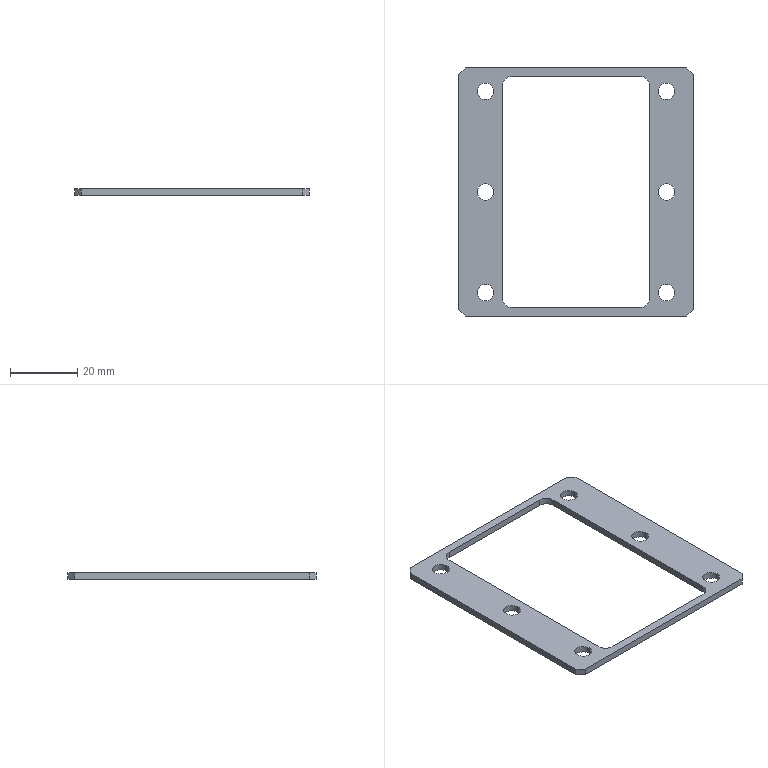Part | SolidWorks | features Chamfer 1, Extrusion 1 | 1 solid | 30 faces | box 70 x 74 x 2 mm | volume 4052 mm3 | cylinder 16 | plane 14 | commonest cylinder face diameters 5 x12 6 x4
STEP:
#1=CARTESIAN_POINT('',(24.5,30.,2.));
#2=VERTEX_POINT('',#1);
#3=CARTESIAN_POINT('',(29.5,30.,2.));
#4=VERTEX_POINT('',#3);
#5=CARTESIAN_POINT('',(27.,30.,2.));
#6=DIRECTION('',(0.,0.,1.));
#7=DIRECTION('',(1.,0.,0.));
#8=AXIS2_PLACEMENT_3D('',#5,#6,#7);
#9=CIRCLE('',#8,2.5);
#10=EDGE_CURVE('',#2,#4,#9,.T.);
#11=ORIENTED_EDGE('',*,*,#10,.T.);
#12=CARTESIAN_POINT('',(29.5,30.,0.));
#13=VERTEX_POINT('',#12);
#14=CARTESIAN_POINT('',(29.5,30.,2.));
#15=DIRECTION('',(0.,0.,-1.));
#16=VECTOR('',#15,1000.);
#17=LINE('',#14,#16);
#18=EDGE_CURVE('',#4,#13,#17,.T.);
#19=ORIENTED_EDGE('',*,*,#18,.T.);
#20=CARTESIAN_POINT('',(24.5,30.,0.));
#21=VERTEX_POINT('',#20);
#22=CARTESIAN_POINT('',(27.,30.,0.));
#23=DIRECTION('',(0.,0.,1.));
#24=DIRECTION('',(1.,0.,0.));
#25=AXIS2_PLACEMENT_3D('',#22,#23,#24);
#26=CIRCLE('',#25,2.5);
#27=EDGE_CURVE('',#21,#13,#26,.T.);
#28=ORIENTED_EDGE('',*,*,#27,.F.);
#29=CARTESIAN_POINT('',(24.5,30.,2.));
#30=DIRECTION('',(0.,0.,-1.));
#31=VECTOR('',#30,1000.);
#32=LINE('',#29,#31);
#33=EDGE_CURVE('',#2,#21,#32,.T.);
#34=ORIENTED_EDGE('',*,*,#33,.F.);
#35=EDGE_LOOP('',(#11,#19,#28,#34));
#36=FACE_OUTER_BOUND('',#35,.T.);
#37=CARTESIAN_POINT('',(27.,30.,2.));
#38=DIRECTION('',(0.,0.,-1.));
#39=DIRECTION('',(-1.,0.,0.));
#40=AXIS2_PLACEMENT_3D('',#37,#38,#39);
#41=CYLINDRICAL_SURFACE('',#40,2.5);
#42=ADVANCED_FACE('',(#36),#41,.F.);
#43=CARTESIAN_POINT('',(24.5,0.,2.));
#44=VERTEX_POINT('',#43);
#45=CARTESIAN_POINT('',(29.5,0.,2.));
#46=VERTEX_POINT('',#45);
#47=CARTESIAN_POINT('',(27.,0.,2.));
#48=DIRECTION('',(0.,0.,1.));
#49=DIRECTION('',(1.,0.,0.));
#50=AXIS2_PLACEMENT_3D('',#47,#48,#49);
#51=CIRCLE('',#50,2.5);
#52=EDGE_CURVE('',#44,#46,#51,.T.);
#53=ORIENTED_EDGE('',*,*,#52,.T.);
#54=CARTESIAN_POINT('',(29.5,0.,0.));
#55=VERTEX_POINT('',#54);
#56=CARTESIAN_POINT('',(29.5,0.,2.));
#57=DIRECTION('',(0.,0.,-1.));
#58=VECTOR('',#57,1000.);
#59=LINE('',#56,#58);
#60=EDGE_CURVE('',#46,#55,#59,.T.);
#61=ORIENTED_EDGE('',*,*,#60,.T.);
#62=CARTESIAN_POINT('',(24.5,0.,0.));
#63=VERTEX_POINT('',#62);
#64=CARTESIAN_POINT('',(27.,0.,0.));
#65=DIRECTION('',(0.,0.,1.));
#66=DIRECTION('',(1.,0.,0.));
#67=AXIS2_PLACEMENT_3D('',#64,#65,#66);
#68=CIRCLE('',#67,2.5);
#69=EDGE_CURVE('',#63,#55,#68,.T.);
#70=ORIENTED_EDGE('',*,*,#69,.F.);
#71=CARTESIAN_POINT('',(24.5,0.,2.));
#72=DIRECTION('',(0.,0.,-1.));
#73=VECTOR('',#72,1000.);
#74=LINE('',#71,#73);
#75=EDGE_CURVE('',#44,#63,#74,.T.);
#76=ORIENTED_EDGE('',*,*,#75,.F.);
#77=EDGE_LOOP('',(#53,#61,#70,#76));
#78=FACE_OUTER_BOUND('',#77,.T.);
#79=CARTESIAN_POINT('',(27.,0.,2.));
#80=DIRECTION('',(0.,0.,-1.));
#81=DIRECTION('',(-1.,0.,0.));
#82=AXIS2_PLACEMENT_3D('',#79,#80,#81);
#83=CYLINDRICAL_SURFACE('',#82,2.5);
#84=ADVANCED_FACE('',(#78),#83,.F.);
#85=CARTESIAN_POINT('',(24.5,-30.,2.));
#86=VERTEX_POINT('',#85);
#87=CARTESIAN_POINT('',(29.5,-30.,2.));
#88=VERTEX_POINT('',#87);
#89=CARTESIAN_POINT('',(27.,-30.,2.));
#90=DIRECTION('',(0.,0.,1.));
#91=DIRECTION('',(1.,0.,0.));
#92=AXIS2_PLACEMENT_3D('',#89,#90,#91);
#93=CIRCLE('',#92,2.5);
#94=EDGE_CURVE('',#86,#88,#93,.T.);
#95=ORIENTED_EDGE('',*,*,#94,.T.);
#96=CARTESIAN_POINT('',(29.5,-30.,0.));
#97=VERTEX_POINT('',#96);
#98=CARTESIAN_POINT('',(29.5,-30.,2.));
#99=DIRECTION('',(0.,0.,-1.));
#100=VECTOR('',#99,1000.);
#101=LINE('',#98,#100);
#102=EDGE_CURVE('',#88,#97,#101,.T.);
#103=ORIENTED_EDGE('',*,*,#102,.T.);
#104=CARTESIAN_POINT('',(24.5,-30.,0.));
#105=VERTEX_POINT('',#104);
#106=CARTESIAN_POINT('',(27.,-30.,0.));
#107=DIRECTION('',(0.,0.,1.));
#108=DIRECTION('',(1.,0.,0.));
#109=AXIS2_PLACEMENT_3D('',#106,#107,#108);
#110=CIRCLE('',#109,2.5);
#111=EDGE_CURVE('',#105,#97,#110,.T.);
#112=ORIENTED_EDGE('',*,*,#111,.F.);
#113=CARTESIAN_POINT('',(24.5,-30.,2.));
#114=DIRECTION('',(0.,0.,-1.));
#115=VECTOR('',#114,1000.);
#116=LINE('',#113,#115);
#117=EDGE_CURVE('',#86,#105,#116,.T.);
#118=ORIENTED_EDGE('',*,*,#117,.F.);
#119=EDGE_LOOP('',(#95,#103,#112,#118));
#120=FACE_OUTER_BOUND('',#119,.T.);
#121=CARTESIAN_POINT('',(27.,-30.,2.));
#122=DIRECTION('',(0.,0.,-1.));
#123=DIRECTION('',(-1.,0.,0.));
#124=AXIS2_PLACEMENT_3D('',#121,#122,#123);
#125=CYLINDRICAL_SURFACE('',#124,2.5);
#126=ADVANCED_FACE('',(#120),#125,.F.);
#127=CARTESIAN_POINT('',(-29.5,-30.,2.));
#128=VERTEX_POINT('',#127);
#129=CARTESIAN_POINT('',(-24.5,-30.,2.));
#130=VERTEX_POINT('',#129);
#131=CARTESIAN_POINT('',(-27.,-30.,2.));
#132=DIRECTION('',(0.,0.,1.));
#133=DIRECTION('',(1.,0.,0.));
#134=AXIS2_PLACEMENT_3D('',#131,#132,#133);
#135=CIRCLE('',#134,2.5);
#136=EDGE_CURVE('',#128,#130,#135,.T.);
#137=ORIENTED_EDGE('',*,*,#136,.T.);
#138=CARTESIAN_POINT('',(-24.5,-30.,0.));
#139=VERTEX_POINT('',#138);
#140=CARTESIAN_POINT('',(-24.5,-30.,2.));
#141=DIRECTION('',(0.,0.,-1.));
#142=VECTOR('',#141,1000.);
#143=LINE('',#140,#142);
#144=EDGE_CURVE('',#130,#139,#143,.T.);
#145=ORIENTED_EDGE('',*,*,#144,.T.);
#146=CARTESIAN_POINT('',(-29.5,-30.,0.));
#147=VERTEX_POINT('',#146);
#148=CARTESIAN_POINT('',(-27.,-30.,0.));
#149=DIRECTION('',(0.,0.,1.));
#150=DIRECTION('',(1.,0.,0.));
#151=AXIS2_PLACEMENT_3D('',#148,#149,#150);
#152=CIRCLE('',#151,2.5);
#153=EDGE_CURVE('',#147,#139,#152,.T.);
#154=ORIENTED_EDGE('',*,*,#153,.F.);
#155=CARTESIAN_POINT('',(-29.5,-30.,2.));
#156=DIRECTION('',(0.,0.,-1.));
#157=VECTOR('',#156,1000.);
#158=LINE('',#155,#157);
#159=EDGE_CURVE('',#128,#147,#158,.T.);
#160=ORIENTED_EDGE('',*,*,#159,.F.);
#161=EDGE_LOOP('',(#137,#145,#154,#160));
#162=FACE_OUTER_BOUND('',#161,.T.);
#163=CARTESIAN_POINT('',(-27.,-30.,2.));
#164=DIRECTION('',(0.,0.,-1.));
#165=DIRECTION('',(-1.,0.,0.));
#166=AXIS2_PLACEMENT_3D('',#163,#164,#165);
#167=CYLINDRICAL_SURFACE('',#166,2.5);
#168=ADVANCED_FACE('',(#162),#167,.F.);
#169=CARTESIAN_POINT('',(-29.5,0.,2.));
#170=VERTEX_POINT('',#169);
#171=CARTESIAN_POINT('',(-24.5,0.,2.));
#172=VERTEX_POINT('',#171);
#173=CARTESIAN_POINT('',(-27.,0.,2.));
#174=DIRECTION('',(0.,0.,1.));
#175=DIRECTION('',(1.,0.,0.));
#176=AXIS2_PLACEMENT_3D('',#173,#174,#175);
#177=CIRCLE('',#176,2.5);
#178=EDGE_CURVE('',#170,#172,#177,.T.);
#179=ORIENTED_EDGE('',*,*,#178,.T.);
#180=CARTESIAN_POINT('',(-24.5,0.,0.));
#181=VERTEX_POINT('',#180);
#182=CARTESIAN_POINT('',(-24.5,0.,2.));
#183=DIRECTION('',(0.,0.,-1.));
#184=VECTOR('',#183,1000.);
#185=LINE('',#182,#184);
#186=EDGE_CURVE('',#172,#181,#185,.T.);
#187=ORIENTED_EDGE('',*,*,#186,.T.);
#188=CARTESIAN_POINT('',(-29.5,0.,0.));
#189=VERTEX_POINT('',#188);
#190=CARTESIAN_POINT('',(-27.,0.,0.));
#191=DIRECTION('',(0.,0.,1.));
#192=DIRECTION('',(1.,0.,0.));
#193=AXIS2_PLACEMENT_3D('',#190,#191,#192);
#194=CIRCLE('',#193,2.5);
#195=EDGE_CURVE('',#189,#181,#194,.T.);
#196=ORIENTED_EDGE('',*,*,#195,.F.);
#197=CARTESIAN_POINT('',(-29.5,0.,2.));
#198=DIRECTION('',(0.,0.,-1.));
#199=VECTOR('',#198,1000.);
#200=LINE('',#197,#199);
#201=EDGE_CURVE('',#170,#189,#200,.T.);
#202=ORIENTED_EDGE('',*,*,#201,.F.);
#203=EDGE_LOOP('',(#179,#187,#196,#202));
#204=FACE_OUTER_BOUND('',#203,.T.);
#205=CARTESIAN_POINT('',(-27.,0.,2.));
#206=DIRECTION('',(0.,0.,-1.));
#207=DIRECTION('',(-1.,0.,0.));
#208=AXIS2_PLACEMENT_3D('',#205,#206,#207);
#209=CYLINDRICAL_SURFACE('',#208,2.5);
#210=ADVANCED_FACE('',(#204),#209,.F.);
#211=CARTESIAN_POINT('',(-29.5,30.,2.));
#212=VERTEX_POINT('',#211);
#213=CARTESIAN_POINT('',(-24.5,30.,2.));
#214=VERTEX_POINT('',#213);
#215=CARTESIAN_POINT('',(-27.,30.,2.));
#216=DIRECTION('',(0.,0.,1.));
#217=DIRECTION('',(1.,0.,0.));
#218=AXIS2_PLACEMENT_3D('',#215,#216,#217);
#219=CIRCLE('',#218,2.5);
#220=EDGE_CURVE('',#212,#214,#219,.T.);
#221=ORIENTED_EDGE('',*,*,#220,.T.);
#222=CARTESIAN_POINT('',(-24.5,30.,0.));
#223=VERTEX_POINT('',#222);
#224=CARTESIAN_POINT('',(-24.5,30.,2.));
#225=DIRECTION('',(0.,0.,-1.));
#226=VECTOR('',#225,1000.);
#227=LINE('',#224,#226);
#228=EDGE_CURVE('',#214,#223,#227,.T.);
#229=ORIENTED_EDGE('',*,*,#228,.T.);
#230=CARTESIAN_POINT('',(-29.5,30.,0.));
#231=VERTEX_POINT('',#230);
#232=CARTESIAN_POINT('',(-27.,30.,0.));
#233=DIRECTION('',(0.,0.,1.));
#234=DIRECTION('',(1.,0.,0.));
#235=AXIS2_PLACEMENT_3D('',#232,#233,#234);
#236=CIRCLE('',#235,2.5);
#237=EDGE_CURVE('',#231,#223,#236,.T.);
#238=ORIENTED_EDGE('',*,*,#237,.F.);
#239=CARTESIAN_POINT('',(-29.5,30.,2.));
#240=DIRECTION('',(0.,0.,-1.));
#241=VECTOR('',#240,1000.);
#242=LINE('',#239,#241);
#243=EDGE_CURVE('',#212,#231,#242,.T.);
#244=ORIENTED_EDGE('',*,*,#243,.F.);
#245=EDGE_LOOP('',(#221,#229,#238,#244));
#246=FACE_OUTER_BOUND('',#245,.T.);
#247=CARTESIAN_POINT('',(-27.,30.,2.));
#248=DIRECTION('',(0.,0.,-1.));
#249=DIRECTION('',(-1.,0.,0.));
#250=AXIS2_PLACEMENT_3D('',#247,#248,#249);
#251=CYLINDRICAL_SURFACE('',#250,2.5);
#252=ADVANCED_FACE('',(#246),#251,.F.);
#253=CARTESIAN_POINT('',(-33.,-37.,2.));
#254=VERTEX_POINT('',#253);
#255=CARTESIAN_POINT('',(33.,-37.,2.));
#256=VERTEX_POINT('',#255);
#257=CARTESIAN_POINT('',(-35.,-37.,2.));
#258=DIRECTION('',(1.,0.,0.));
#259=VECTOR('',#258,1000.);
#260=LINE('',#257,#259);
#261=EDGE_CURVE('',#254,#256,#260,.T.);
#262=ORIENTED_EDGE('',*,*,#261,.T.);
#263=CARTESIAN_POINT('',(35.,-35.,2.));
#264=VERTEX_POINT('',#263);
#265=CARTESIAN_POINT('',(35.,-35.,2.));
#266=DIRECTION('',(0.7071,0.7071,0.));
#267=VECTOR('',#266,1000.);
#268=LINE('',#265,#267);
#269=EDGE_CURVE('',#256,#264,#268,.T.);
#270=ORIENTED_EDGE('',*,*,#269,.T.);
#271=CARTESIAN_POINT('',(35.,35.,2.));
#272=VERTEX_POINT('',#271);
#273=CARTESIAN_POINT('',(35.,-37.,2.));
#274=DIRECTION('',(0.,1.,0.));
#275=VECTOR('',#274,1000.);
#276=LINE('',#273,#275);
#277=EDGE_CURVE('',#264,#272,#276,.T.);
#278=ORIENTED_EDGE('',*,*,#277,.T.);
#279=CARTESIAN_POINT('',(33.,37.,2.));
#280=VERTEX_POINT('',#279);
#281=CARTESIAN_POINT('',(33.,37.,2.));
#282=DIRECTION('',(-0.7071,0.7071,0.));
#283=VECTOR('',#282,1000.);
#284=LINE('',#281,#283);
#285=EDGE_CURVE('',#272,#280,#284,.T.);
#286=ORIENTED_EDGE('',*,*,#285,.T.);
#287=CARTESIAN_POINT('',(-33.,37.,2.));
#288=VERTEX_POINT('',#287);
#289=CARTESIAN_POINT('',(-35.,37.,2.));
#290=DIRECTION('',(-1.,0.,0.));
#291=VECTOR('',#290,1000.);
#292=LINE('',#289,#291);
#293=EDGE_CURVE('',#280,#288,#292,.T.);
#294=ORIENTED_EDGE('',*,*,#293,.T.);
#295=CARTESIAN_POINT('',(-35.,35.,2.));
#296=VERTEX_POINT('',#295);
#297=CARTESIAN_POINT('',(-35.,35.,2.));
#298=DIRECTION('',(-0.7071,-0.7071,0.));
#299=VECTOR('',#298,1000.);
#300=LINE('',#297,#299);
#301=EDGE_CURVE('',#288,#296,#300,.T.);
#302=ORIENTED_EDGE('',*,*,#301,.T.);
#303=CARTESIAN_POINT('',(-35.,-35.,2.));
#304=VERTEX_POINT('',#303);
#305=CARTESIAN_POINT('',(-35.,-37.,2.));
#306=DIRECTION('',(0.,-1.,0.));
#307=VECTOR('',#306,1000.);
#308=LINE('',#305,#307);
#309=EDGE_CURVE('',#296,#304,#308,.T.);
#310=ORIENTED_EDGE('',*,*,#309,.T.);
#311=CARTESIAN_POINT('',(-33.,-37.,2.));
#312=DIRECTION('',(0.7071,-0.7071,0.));
#313=VECTOR('',#312,1000.);
#314=LINE('',#311,#313);
#315=EDGE_CURVE('',#304,#254,#314,.T.);
#316=ORIENTED_EDGE('',*,*,#315,.T.);
#317=EDGE_LOOP('',(#262,#270,#278,#286,#294,#302,#310,#316));
#318=FACE_OUTER_BOUND('',#317,.T.);
#319=CARTESIAN_POINT('',(22.,31.5,2.));
#320=VERTEX_POINT('',#319);
#321=CARTESIAN_POINT('',(19.,34.5,2.));
#322=VERTEX_POINT('',#321);
#323=CARTESIAN_POINT('',(19.,31.5,2.));
#324=DIRECTION('',(0.,0.,1.));
#325=DIRECTION('',(-1.,0.,0.));
#326=AXIS2_PLACEMENT_3D('',#323,#324,#325);
#327=CIRCLE('',#326,3.);
#328=EDGE_CURVE('',#320,#322,#327,.T.);
#329=ORIENTED_EDGE('',*,*,#328,.F.);
#330=CARTESIAN_POINT('',(22.,-31.5,2.));
#331=VERTEX_POINT('',#330);
#332=CARTESIAN_POINT('',(22.,-31.5,2.));
#333=DIRECTION('',(0.,1.,0.));
#334=VECTOR('',#333,1000.);
#335=LINE('',#332,#334);
#336=EDGE_CURVE('',#331,#320,#335,.T.);
#337=ORIENTED_EDGE('',*,*,#336,.F.);
#338=CARTESIAN_POINT('',(19.,-34.5,2.));
#339=VERTEX_POINT('',#338);
#340=CARTESIAN_POINT('',(19.,-31.5,2.));
#341=DIRECTION('',(0.,0.,1.));
#342=DIRECTION('',(-1.,0.,0.));
#343=AXIS2_PLACEMENT_3D('',#340,#341,#342);
#344=CIRCLE('',#343,3.);
#345=EDGE_CURVE('',#339,#331,#344,.T.);
#346=ORIENTED_EDGE('',*,*,#345,.F.);
#347=CARTESIAN_POINT('',(-19.,-34.5,2.));
#348=VERTEX_POINT('',#347);
#349=CARTESIAN_POINT('',(-19.,-34.5,2.));
#350=DIRECTION('',(1.,0.,0.));
#351=VECTOR('',#350,1000.);
#352=LINE('',#349,#351);
#353=EDGE_CURVE('',#348,#339,#352,.T.);
#354=ORIENTED_EDGE('',*,*,#353,.F.);
#355=CARTESIAN_POINT('',(-22.,-31.5,2.));
#356=VERTEX_POINT('',#355);
#357=CARTESIAN_POINT('',(-19.,-31.5,2.));
#358=DIRECTION('',(0.,0.,1.));
#359=DIRECTION('',(-1.,0.,0.));
#360=AXIS2_PLACEMENT_3D('',#357,#358,#359);
#361=CIRCLE('',#360,3.);
#362=EDGE_CURVE('',#356,#348,#361,.T.);
#363=ORIENTED_EDGE('',*,*,#362,.F.);
#364=CARTESIAN_POINT('',(-22.,31.5,2.));
#365=VERTEX_POINT('',#364);
#366=CARTESIAN_POINT('',(-22.,-31.5,2.));
#367=DIRECTION('',(0.,-1.,0.));
#368=VECTOR('',#367,1000.);
#369=LINE('',#366,#368);
#370=EDGE_CURVE('',#365,#356,#369,.T.);
#371=ORIENTED_EDGE('',*,*,#370,.F.);
#372=CARTESIAN_POINT('',(-19.,34.5,2.));
#373=VERTEX_POINT('',#372);
#374=CARTESIAN_POINT('',(-19.,31.5,2.));
#375=DIRECTION('',(0.,0.,1.));
#376=DIRECTION('',(-1.,0.,0.));
#377=AXIS2_PLACEMENT_3D('',#374,#375,#376);
#378=CIRCLE('',#377,3.);
#379=EDGE_CURVE('',#373,#365,#378,.T.);
#380=ORIENTED_EDGE('',*,*,#379,.F.);
#381=CARTESIAN_POINT('',(-19.,34.5,2.));
#382=DIRECTION('',(-1.,0.,0.));
#383=VECTOR('',#382,1000.);
#384=LINE('',#381,#383);
#385=EDGE_CURVE('',#322,#373,#384,.T.);
#386=ORIENTED_EDGE('',*,*,#385,.F.);
#387=EDGE_LOOP('',(#329,#337,#346,#354,#363,#371,#380,#386));
#388=FACE_BOUND('',#387,.T.);
#389=ORIENTED_EDGE('',*,*,#220,.F.);
#390=CARTESIAN_POINT('',(-27.,30.,2.));
#391=DIRECTION('',(0.,0.,1.));
#392=DIRECTION('',(1.,0.,0.));
#393=AXIS2_PLACEMENT_3D('',#390,#391,#392);
#394=CIRCLE('',#393,2.5);
#395=EDGE_CURVE('',#214,#212,#394,.T.);
#396=ORIENTED_EDGE('',*,*,#395,.F.);
#397=EDGE_LOOP('',(#389,#396));
#398=FACE_BOUND('',#397,.T.);
#399=ORIENTED_EDGE('',*,*,#178,.F.);
#400=CARTESIAN_POINT('',(-27.,0.,2.));
#401=DIRECTION('',(0.,0.,1.));
#402=DIRECTION('',(1.,0.,0.));
#403=AXIS2_PLACEMENT_3D('',#400,#401,#402);
#404=CIRCLE('',#403,2.5);
#405=EDGE_CURVE('',#172,#170,#404,.T.);
#406=ORIENTED_EDGE('',*,*,#405,.F.);
#407=EDGE_LOOP('',(#399,#406));
#408=FACE_BOUND('',#407,.T.);
#409=ORIENTED_EDGE('',*,*,#136,.F.);
#410=CARTESIAN_POINT('',(-27.,-30.,2.));
#411=DIRECTION('',(0.,0.,1.));
#412=DIRECTION('',(1.,0.,0.));
#413=AXIS2_PLACEMENT_3D('',#410,#411,#412);
#414=CIRCLE('',#413,2.5);
#415=EDGE_CURVE('',#130,#128,#414,.T.);
#416=ORIENTED_EDGE('',*,*,#415,.F.);
#417=EDGE_LOOP('',(#409,#416));
#418=FACE_BOUND('',#417,.T.);
#419=ORIENTED_EDGE('',*,*,#94,.F.);
#420=CARTESIAN_POINT('',(27.,-30.,2.));
#421=DIRECTION('',(0.,0.,1.));
#422=DIRECTION('',(1.,0.,0.));
#423=AXIS2_PLACEMENT_3D('',#420,#421,#422);
#424=CIRCLE('',#423,2.5);
#425=EDGE_CURVE('',#88,#86,#424,.T.);
#426=ORIENTED_EDGE('',*,*,#425,.F.);
#427=EDGE_LOOP('',(#419,#426));
#428=FACE_BOUND('',#427,.T.);
#429=ORIENTED_EDGE('',*,*,#52,.F.);
#430=CARTESIAN_POINT('',(27.,0.,2.));
#431=DIRECTION('',(0.,0.,1.));
#432=DIRECTION('',(1.,0.,0.));
#433=AXIS2_PLACEMENT_3D('',#430,#431,#432);
#434=CIRCLE('',#433,2.5);
#435=EDGE_CURVE('',#46,#44,#434,.T.);
#436=ORIENTED_EDGE('',*,*,#435,.F.);
#437=EDGE_LOOP('',(#429,#436));
#438=FACE_BOUND('',#437,.T.);
#439=ORIENTED_EDGE('',*,*,#10,.F.);
#440=CARTESIAN_POINT('',(27.,30.,2.));
#441=DIRECTION('',(0.,0.,1.));
#442=DIRECTION('',(1.,0.,0.));
#443=AXIS2_PLACEMENT_3D('',#440,#441,#442);
#444=CIRCLE('',#443,2.5);
#445=EDGE_CURVE('',#4,#2,#444,.T.);
#446=ORIENTED_EDGE('',*,*,#445,.F.);
#447=EDGE_LOOP('',(#439,#446));
#448=FACE_BOUND('',#447,.T.);
#449=CARTESIAN_POINT('',(0.,0.,2.));
#450=DIRECTION('',(0.,0.,-1.));
#451=DIRECTION('',(-1.,0.,0.));
#452=AXIS2_PLACEMENT_3D('',#449,#450,#451);
#453=PLANE('',#452);
#454=ADVANCED_FACE('',(#318,#388,#398,#408,#418,#428,#438,#448),#453,.F.);
#455=ORIENTED_EDGE('',*,*,#69,.T.);
#456=CARTESIAN_POINT('',(27.,0.,0.));
#457=DIRECTION('',(0.,0.,1.));
#458=DIRECTION('',(1.,0.,0.));
#459=AXIS2_PLACEMENT_3D('',#456,#457,#458);
#460=CIRCLE('',#459,2.5);
#461=EDGE_CURVE('',#55,#63,#460,.T.);
#462=ORIENTED_EDGE('',*,*,#461,.T.);
#463=EDGE_LOOP('',(#455,#462));
#464=FACE_BOUND('',#463,.T.);
#465=ORIENTED_EDGE('',*,*,#153,.T.);
#466=CARTESIAN_POINT('',(-27.,-30.,0.));
#467=DIRECTION('',(0.,0.,1.));
#468=DIRECTION('',(1.,0.,0.));
#469=AXIS2_PLACEMENT_3D('',#466,#467,#468);
#470=CIRCLE('',#469,2.5);
#471=EDGE_CURVE('',#139,#147,#470,.T.);
#472=ORIENTED_EDGE('',*,*,#471,.T.);
#473=EDGE_LOOP('',(#465,#472));
#474=FACE_BOUND('',#473,.T.);
#475=ORIENTED_EDGE('',*,*,#237,.T.);
#476=CARTESIAN_POINT('',(-27.,30.,0.));
#477=DIRECTION('',(0.,0.,1.));
#478=DIRECTION('',(1.,0.,0.));
#479=AXIS2_PLACEMENT_3D('',#476,#477,#478);
#480=CIRCLE('',#479,2.5);
#481=EDGE_CURVE('',#223,#231,#480,.T.);
#482=ORIENTED_EDGE('',*,*,#481,.T.);
#483=EDGE_LOOP('',(#475,#482));
#484=FACE_BOUND('',#483,.T.);
#485=CARTESIAN_POINT('',(35.,-35.,0.));
#486=VERTEX_POINT('',#485);
#487=CARTESIAN_POINT('',(35.,35.,0.));
#488=VERTEX_POINT('',#487);
#489=CARTESIAN_POINT('',(35.,-37.,0.));
#490=DIRECTION('',(0.,1.,0.));
#491=VECTOR('',#490,1000.);
#492=LINE('',#489,#491);
#493=EDGE_CURVE('',#486,#488,#492,.T.);
#494=ORIENTED_EDGE('',*,*,#493,.F.);
#495=CARTESIAN_POINT('',(33.,-37.,0.));
#496=VERTEX_POINT('',#495);
#497=CARTESIAN_POINT('',(35.,-35.,0.));
#498=DIRECTION('',(-0.7071,-0.7071,0.));
#499=VECTOR('',#498,1000.);
#500=LINE('',#497,#499);
#501=EDGE_CURVE('',#486,#496,#500,.T.);
#502=ORIENTED_EDGE('',*,*,#501,.T.);
#503=CARTESIAN_POINT('',(-33.,-37.,0.));
#504=VERTEX_POINT('',#503);
#505=CARTESIAN_POINT('',(-35.,-37.,0.));
#506=DIRECTION('',(1.,0.,0.));
#507=VECTOR('',#506,1000.);
#508=LINE('',#505,#507);
#509=EDGE_CURVE('',#504,#496,#508,.T.);
#510=ORIENTED_EDGE('',*,*,#509,.F.);
#511=CARTESIAN_POINT('',(-35.,-35.,0.));
#512=VERTEX_POINT('',#511);
#513=CARTESIAN_POINT('',(-35.,-35.,0.));
#514=DIRECTION('',(-0.7071,0.7071,0.));
#515=VECTOR('',#514,1000.);
#516=LINE('',#513,#515);
#517=EDGE_CURVE('',#504,#512,#516,.T.);
#518=ORIENTED_EDGE('',*,*,#517,.T.);
#519=CARTESIAN_POINT('',(-35.,35.,0.));
#520=VERTEX_POINT('',#519);
#521=CARTESIAN_POINT('',(-35.,-37.,0.));
#522=DIRECTION('',(0.,-1.,0.));
#523=VECTOR('',#522,1000.);
#524=LINE('',#521,#523);
#525=EDGE_CURVE('',#520,#512,#524,.T.);
#526=ORIENTED_EDGE('',*,*,#525,.F.);
#527=CARTESIAN_POINT('',(-33.,37.,0.));
#528=VERTEX_POINT('',#527);
#529=CARTESIAN_POINT('',(-35.,35.,0.));
#530=DIRECTION('',(0.7071,0.7071,0.));
#531=VECTOR('',#530,1000.);
#532=LINE('',#529,#531);
#533=EDGE_CURVE('',#520,#528,#532,.T.);
#534=ORIENTED_EDGE('',*,*,#533,.T.);
#535=CARTESIAN_POINT('',(33.,37.,0.));
#536=VERTEX_POINT('',#535);
#537=CARTESIAN_POINT('',(-35.,37.,0.));
#538=DIRECTION('',(-1.,0.,0.));
#539=VECTOR('',#538,1000.);
#540=LINE('',#537,#539);
#541=EDGE_CURVE('',#536,#528,#540,.T.);
#542=ORIENTED_EDGE('',*,*,#541,.F.);
#543=CARTESIAN_POINT('',(35.,35.,0.));
#544=DIRECTION('',(0.7071,-0.7071,0.));
#545=VECTOR('',#544,1000.);
#546=LINE('',#543,#545);
#547=EDGE_CURVE('',#536,#488,#546,.T.);
#548=ORIENTED_EDGE('',*,*,#547,.T.);
#549=EDGE_LOOP('',(#494,#502,#510,#518,#526,#534,#542,#548));
#550=FACE_OUTER_BOUND('',#549,.T.);
#551=CARTESIAN_POINT('',(22.,-31.5,0.));
#552=VERTEX_POINT('',#551);
#553=CARTESIAN_POINT('',(22.,31.5,0.));
#554=VERTEX_POINT('',#553);
#555=CARTESIAN_POINT('',(22.,-31.5,0.));
#556=DIRECTION('',(0.,1.,0.));
#557=VECTOR('',#556,1000.);
#558=LINE('',#555,#557);
#559=EDGE_CURVE('',#552,#554,#558,.T.);
#560=ORIENTED_EDGE('',*,*,#559,.T.);
#561=CARTESIAN_POINT('',(19.,34.5,0.));
#562=VERTEX_POINT('',#561);
#563=CARTESIAN_POINT('',(19.,31.5,0.));
#564=DIRECTION('',(0.,0.,1.));
#565=DIRECTION('',(-1.,0.,0.));
#566=AXIS2_PLACEMENT_3D('',#563,#564,#565);
#567=CIRCLE('',#566,3.);
#568=EDGE_CURVE('',#554,#562,#567,.T.);
#569=ORIENTED_EDGE('',*,*,#568,.T.);
#570=CARTESIAN_POINT('',(-19.,34.5,0.));
#571=VERTEX_POINT('',#570);
#572=CARTESIAN_POINT('',(-19.,34.5,0.));
#573=DIRECTION('',(-1.,0.,0.));
#574=VECTOR('',#573,1000.);
#575=LINE('',#572,#574);
#576=EDGE_CURVE('',#562,#571,#575,.T.);
#577=ORIENTED_EDGE('',*,*,#576,.T.);
#578=CARTESIAN_POINT('',(-22.,31.5,0.));
#579=VERTEX_POINT('',#578);
#580=CARTESIAN_POINT('',(-19.,31.5,0.));
#581=DIRECTION('',(0.,0.,1.));
#582=DIRECTION('',(-1.,0.,0.));
#583=AXIS2_PLACEMENT_3D('',#580,#581,#582);
#584=CIRCLE('',#583,3.);
#585=EDGE_CURVE('',#571,#579,#584,.T.);
#586=ORIENTED_EDGE('',*,*,#585,.T.);
#587=CARTESIAN_POINT('',(-22.,-31.5,0.));
#588=VERTEX_POINT('',#587);
#589=CARTESIAN_POINT('',(-22.,-31.5,0.));
#590=DIRECTION('',(0.,-1.,0.));
#591=VECTOR('',#590,1000.);
#592=LINE('',#589,#591);
#593=EDGE_CURVE('',#579,#588,#592,.T.);
#594=ORIENTED_EDGE('',*,*,#593,.T.);
#595=CARTESIAN_POINT('',(-19.,-34.5,0.));
#596=VERTEX_POINT('',#595);
#597=CARTESIAN_POINT('',(-19.,-31.5,0.));
#598=DIRECTION('',(0.,0.,1.));
#599=DIRECTION('',(-1.,0.,0.));
#600=AXIS2_PLACEMENT_3D('',#597,#598,#599);
#601=CIRCLE('',#600,3.);
#602=EDGE_CURVE('',#588,#596,#601,.T.);
#603=ORIENTED_EDGE('',*,*,#602,.T.);
#604=CARTESIAN_POINT('',(19.,-34.5,0.));
#605=VERTEX_POINT('',#604);
#606=CARTESIAN_POINT('',(-19.,-34.5,0.));
#607=DIRECTION('',(1.,0.,0.));
#608=VECTOR('',#607,1000.);
#609=LINE('',#606,#608);
#610=EDGE_CURVE('',#596,#605,#609,.T.);
#611=ORIENTED_EDGE('',*,*,#610,.T.);
#612=CARTESIAN_POINT('',(19.,-31.5,0.));
#613=DIRECTION('',(0.,0.,1.));
#614=DIRECTION('',(-1.,0.,0.));
#615=AXIS2_PLACEMENT_3D('',#612,#613,#614);
#616=CIRCLE('',#615,3.);
#617=EDGE_CURVE('',#605,#552,#616,.T.);
#618=ORIENTED_EDGE('',*,*,#617,.T.);
#619=EDGE_LOOP('',(#560,#569,#577,#586,#594,#603,#611,#618));
#620=FACE_BOUND('',#619,.T.);
#621=ORIENTED_EDGE('',*,*,#195,.T.);
#622=CARTESIAN_POINT('',(-27.,0.,0.));
#623=DIRECTION('',(0.,0.,1.));
#624=DIRECTION('',(1.,0.,0.));
#625=AXIS2_PLACEMENT_3D('',#622,#623,#624);
#626=CIRCLE('',#625,2.5);
#627=EDGE_CURVE('',#181,#189,#626,.T.);
#628=ORIENTED_EDGE('',*,*,#627,.T.);
#629=EDGE_LOOP('',(#621,#628));
#630=FACE_BOUND('',#629,.T.);
#631=ORIENTED_EDGE('',*,*,#111,.T.);
#632=CARTESIAN_POINT('',(27.,-30.,0.));
#633=DIRECTION('',(0.,0.,1.));
#634=DIRECTION('',(1.,0.,0.));
#635=AXIS2_PLACEMENT_3D('',#632,#633,#634);
#636=CIRCLE('',#635,2.5);
#637=EDGE_CURVE('',#97,#105,#636,.T.);
#638=ORIENTED_EDGE('',*,*,#637,.T.);
#639=EDGE_LOOP('',(#631,#638));
#640=FACE_BOUND('',#639,.T.);
#641=ORIENTED_EDGE('',*,*,#27,.T.);
#642=CARTESIAN_POINT('',(27.,30.,0.));
#643=DIRECTION('',(0.,0.,1.));
#644=DIRECTION('',(1.,0.,0.));
#645=AXIS2_PLACEMENT_3D('',#642,#643,#644);
#646=CIRCLE('',#645,2.5);
#647=EDGE_CURVE('',#13,#21,#646,.T.);
#648=ORIENTED_EDGE('',*,*,#647,.T.);
#649=EDGE_LOOP('',(#641,#648));
#650=FACE_BOUND('',#649,.T.);
#651=CARTESIAN_POINT('',(0.,0.,0.));
#652=DIRECTION('',(0.,0.,-1.));
#653=DIRECTION('',(-1.,0.,0.));
#654=AXIS2_PLACEMENT_3D('',#651,#652,#653);
#655=PLANE('',#654);
#656=ADVANCED_FACE('',(#464,#474,#484,#550,#620,#630,#640,#650),#655,.T.);
#657=ORIENTED_EDGE('',*,*,#277,.F.);
#658=CARTESIAN_POINT('',(35.,-35.,2.));
#659=DIRECTION('',(0.,0.,-1.));
#660=VECTOR('',#659,1000.);
#661=LINE('',#658,#660);
#662=EDGE_CURVE('',#264,#486,#661,.T.);
#663=ORIENTED_EDGE('',*,*,#662,.T.);
#664=ORIENTED_EDGE('',*,*,#493,.T.);
#665=CARTESIAN_POINT('',(35.,35.,2.));
#666=DIRECTION('',(0.,0.,1.));
#667=VECTOR('',#666,1000.);
#668=LINE('',#665,#667);
#669=EDGE_CURVE('',#488,#272,#668,.T.);
#670=ORIENTED_EDGE('',*,*,#669,.T.);
#671=EDGE_LOOP('',(#657,#663,#664,#670));
#672=FACE_OUTER_BOUND('',#671,.T.);
#673=CARTESIAN_POINT('',(35.,-37.,2.));
#674=DIRECTION('',(-1.,0.,0.));
#675=DIRECTION('',(0.,0.,1.));
#676=AXIS2_PLACEMENT_3D('',#673,#674,#675);
#677=PLANE('',#676);
#678=ADVANCED_FACE('',(#672),#677,.F.);
#679=ORIENTED_EDGE('',*,*,#293,.F.);
#680=CARTESIAN_POINT('',(33.,37.,2.));
#681=DIRECTION('',(0.,0.,-1.));
#682=VECTOR('',#681,1000.);
#683=LINE('',#680,#682);
#684=EDGE_CURVE('',#280,#536,#683,.T.);
#685=ORIENTED_EDGE('',*,*,#684,.T.);
#686=ORIENTED_EDGE('',*,*,#541,.T.);
#687=CARTESIAN_POINT('',(-33.,37.,2.));
#688=DIRECTION('',(0.,0.,1.));
#689=VECTOR('',#688,1000.);
#690=LINE('',#687,#689);
#691=EDGE_CURVE('',#528,#288,#690,.T.);
#692=ORIENTED_EDGE('',*,*,#691,.T.);
#693=EDGE_LOOP('',(#679,#685,#686,#692));
#694=FACE_OUTER_BOUND('',#693,.T.);
#695=CARTESIAN_POINT('',(-35.,37.,2.));
#696=DIRECTION('',(0.,-1.,0.));
#697=DIRECTION('',(0.,0.,-1.));
#698=AXIS2_PLACEMENT_3D('',#695,#696,#697);
#699=PLANE('',#698);
#700=ADVANCED_FACE('',(#694),#699,.F.);
#701=ORIENTED_EDGE('',*,*,#525,.T.);
#702=CARTESIAN_POINT('',(-35.,-35.,2.));
#703=DIRECTION('',(0.,0.,1.));
#704=VECTOR('',#703,1000.);
#705=LINE('',#702,#704);
#706=EDGE_CURVE('',#512,#304,#705,.T.);
#707=ORIENTED_EDGE('',*,*,#706,.T.);
#708=ORIENTED_EDGE('',*,*,#309,.F.);
#709=CARTESIAN_POINT('',(-35.,35.,2.));
#710=DIRECTION('',(0.,0.,-1.));
#711=VECTOR('',#710,1000.);
#712=LINE('',#709,#711);
#713=EDGE_CURVE('',#296,#520,#712,.T.);
#714=ORIENTED_EDGE('',*,*,#713,.T.);
#715=EDGE_LOOP('',(#701,#707,#708,#714));
#716=FACE_OUTER_BOUND('',#715,.T.);
#717=CARTESIAN_POINT('',(-35.,-37.,2.));
#718=DIRECTION('',(1.,0.,0.));
#719=DIRECTION('',(0.,0.,-1.));
#720=AXIS2_PLACEMENT_3D('',#717,#718,#719);
#721=PLANE('',#720);
#722=ADVANCED_FACE('',(#716),#721,.F.);
#723=ORIENTED_EDGE('',*,*,#509,.T.);
#724=CARTESIAN_POINT('',(33.,-37.,2.));
#725=DIRECTION('',(0.,0.,1.));
#726=VECTOR('',#725,1000.);
#727=LINE('',#724,#726);
#728=EDGE_CURVE('',#496,#256,#727,.T.);
#729=ORIENTED_EDGE('',*,*,#728,.T.);
#730=ORIENTED_EDGE('',*,*,#261,.F.);
#731=CARTESIAN_POINT('',(-33.,-37.,2.));
#732=DIRECTION('',(0.,0.,-1.));
#733=VECTOR('',#732,1000.);
#734=LINE('',#731,#733);
#735=EDGE_CURVE('',#254,#504,#734,.T.);
#736=ORIENTED_EDGE('',*,*,#735,.T.);
#737=EDGE_LOOP('',(#723,#729,#730,#736));
#738=FACE_OUTER_BOUND('',#737,.T.);
#739=CARTESIAN_POINT('',(-35.,-37.,2.));
#740=DIRECTION('',(0.,1.,0.));
#741=DIRECTION('',(0.,0.,1.));
#742=AXIS2_PLACEMENT_3D('',#739,#740,#741);
#743=PLANE('',#742);
#744=ADVANCED_FACE('',(#738),#743,.F.);
#745=ORIENTED_EDGE('',*,*,#568,.F.);
#746=CARTESIAN_POINT('',(22.,31.5,2.));
#747=DIRECTION('',(0.,0.,-1.));
#748=VECTOR('',#747,1000.);
#749=LINE('',#746,#748);
#750=EDGE_CURVE('',#320,#554,#749,.T.);
#751=ORIENTED_EDGE('',*,*,#750,.F.);
#752=ORIENTED_EDGE('',*,*,#328,.T.);
#753=CARTESIAN_POINT('',(19.,34.5,2.));
#754=DIRECTION('',(0.,0.,-1.));
#755=VECTOR('',#754,1000.);
#756=LINE('',#753,#755);
#757=EDGE_CURVE('',#322,#562,#756,.T.);
#758=ORIENTED_EDGE('',*,*,#757,.T.);
#759=EDGE_LOOP('',(#745,#751,#752,#758));
#760=FACE_OUTER_BOUND('',#759,.T.);
#761=CARTESIAN_POINT('',(19.,31.5,2.));
#762=DIRECTION('',(0.,0.,-1.));
#763=DIRECTION('',(-1.,0.,0.));
#764=AXIS2_PLACEMENT_3D('',#761,#762,#763);
#765=CYLINDRICAL_SURFACE('',#764,3.);
#766=ADVANCED_FACE('',(#760),#765,.F.);
#767=ORIENTED_EDGE('',*,*,#576,.F.);
#768=ORIENTED_EDGE('',*,*,#757,.F.);
#769=ORIENTED_EDGE('',*,*,#385,.T.);
#770=CARTESIAN_POINT('',(-19.,34.5,2.));
#771=DIRECTION('',(0.,0.,-1.));
#772=VECTOR('',#771,1000.);
#773=LINE('',#770,#772);
#774=EDGE_CURVE('',#373,#571,#773,.T.);
#775=ORIENTED_EDGE('',*,*,#774,.T.);
#776=EDGE_LOOP('',(#767,#768,#769,#775));
#777=FACE_OUTER_BOUND('',#776,.T.);
#778=CARTESIAN_POINT('',(-19.,34.5,2.));
#779=DIRECTION('',(0.,-1.,0.));
#780=DIRECTION('',(0.,0.,-1.));
#781=AXIS2_PLACEMENT_3D('',#778,#779,#780);
#782=PLANE('',#781);
#783=ADVANCED_FACE('',(#777),#782,.T.);
#784=ORIENTED_EDGE('',*,*,#585,.F.);
#785=ORIENTED_EDGE('',*,*,#774,.F.);
#786=ORIENTED_EDGE('',*,*,#379,.T.);
#787=CARTESIAN_POINT('',(-22.,31.5,2.));
#788=DIRECTION('',(0.,0.,-1.));
#789=VECTOR('',#788,1000.);
#790=LINE('',#787,#789);
#791=EDGE_CURVE('',#365,#579,#790,.T.);
#792=ORIENTED_EDGE('',*,*,#791,.T.);
#793=EDGE_LOOP('',(#784,#785,#786,#792));
#794=FACE_OUTER_BOUND('',#793,.T.);
#795=CARTESIAN_POINT('',(-19.,31.5,2.));
#796=DIRECTION('',(0.,0.,-1.));
#797=DIRECTION('',(-1.,0.,0.));
#798=AXIS2_PLACEMENT_3D('',#795,#796,#797);
#799=CYLINDRICAL_SURFACE('',#798,3.);
#800=ADVANCED_FACE('',(#794),#799,.F.);
#801=ORIENTED_EDGE('',*,*,#593,.F.);
#802=ORIENTED_EDGE('',*,*,#791,.F.);
#803=ORIENTED_EDGE('',*,*,#370,.T.);
#804=CARTESIAN_POINT('',(-22.,-31.5,2.));
#805=DIRECTION('',(0.,0.,-1.));
#806=VECTOR('',#805,1000.);
#807=LINE('',#804,#806);
#808=EDGE_CURVE('',#356,#588,#807,.T.);
#809=ORIENTED_EDGE('',*,*,#808,.T.);
#810=EDGE_LOOP('',(#801,#802,#803,#809));
#811=FACE_OUTER_BOUND('',#810,.T.);
#812=CARTESIAN_POINT('',(-22.,-31.5,2.));
#813=DIRECTION('',(1.,0.,0.));
#814=DIRECTION('',(0.,0.,-1.));
#815=AXIS2_PLACEMENT_3D('',#812,#813,#814);
#816=PLANE('',#815);
#817=ADVANCED_FACE('',(#811),#816,.T.);
#818=ORIENTED_EDGE('',*,*,#602,.F.);
#819=ORIENTED_EDGE('',*,*,#808,.F.);
#820=ORIENTED_EDGE('',*,*,#362,.T.);
#821=CARTESIAN_POINT('',(-19.,-34.5,2.));
#822=DIRECTION('',(0.,0.,-1.));
#823=VECTOR('',#822,1000.);
#824=LINE('',#821,#823);
#825=EDGE_CURVE('',#348,#596,#824,.T.);
#826=ORIENTED_EDGE('',*,*,#825,.T.);
#827=EDGE_LOOP('',(#818,#819,#820,#826));
#828=FACE_OUTER_BOUND('',#827,.T.);
#829=CARTESIAN_POINT('',(-19.,-31.5,2.));
#830=DIRECTION('',(0.,0.,-1.));
#831=DIRECTION('',(-1.,0.,0.));
#832=AXIS2_PLACEMENT_3D('',#829,#830,#831);
#833=CYLINDRICAL_SURFACE('',#832,3.);
#834=ADVANCED_FACE('',(#828),#833,.F.);
#835=ORIENTED_EDGE('',*,*,#610,.F.);
#836=ORIENTED_EDGE('',*,*,#825,.F.);
#837=ORIENTED_EDGE('',*,*,#353,.T.);
#838=CARTESIAN_POINT('',(19.,-34.5,2.));
#839=DIRECTION('',(0.,0.,-1.));
#840=VECTOR('',#839,1000.);
#841=LINE('',#838,#840);
#842=EDGE_CURVE('',#339,#605,#841,.T.);
#843=ORIENTED_EDGE('',*,*,#842,.T.);
#844=EDGE_LOOP('',(#835,#836,#837,#843));
#845=FACE_OUTER_BOUND('',#844,.T.);
#846=CARTESIAN_POINT('',(-19.,-34.5,2.));
#847=DIRECTION('',(0.,1.,0.));
#848=DIRECTION('',(0.,0.,1.));
#849=AXIS2_PLACEMENT_3D('',#846,#847,#848);
#850=PLANE('',#849);
#851=ADVANCED_FACE('',(#845),#850,.T.);
#852=ORIENTED_EDGE('',*,*,#617,.F.);
#853=ORIENTED_EDGE('',*,*,#842,.F.);
#854=ORIENTED_EDGE('',*,*,#345,.T.);
#855=CARTESIAN_POINT('',(22.,-31.5,2.));
#856=DIRECTION('',(0.,0.,-1.));
#857=VECTOR('',#856,1000.);
#858=LINE('',#855,#857);
#859=EDGE_CURVE('',#331,#552,#858,.T.);
#860=ORIENTED_EDGE('',*,*,#859,.T.);
#861=EDGE_LOOP('',(#852,#853,#854,#860));
#862=FACE_OUTER_BOUND('',#861,.T.);
#863=CARTESIAN_POINT('',(19.,-31.5,2.));
#864=DIRECTION('',(0.,0.,-1.));
#865=DIRECTION('',(-1.,0.,0.));
#866=AXIS2_PLACEMENT_3D('',#863,#864,#865);
#867=CYLINDRICAL_SURFACE('',#866,3.);
#868=ADVANCED_FACE('',(#862),#867,.F.);
#869=ORIENTED_EDGE('',*,*,#559,.F.);
#870=ORIENTED_EDGE('',*,*,#859,.F.);
#871=ORIENTED_EDGE('',*,*,#336,.T.);
#872=ORIENTED_EDGE('',*,*,#750,.T.);
#873=EDGE_LOOP('',(#869,#870,#871,#872));
#874=FACE_OUTER_BOUND('',#873,.T.);
#875=CARTESIAN_POINT('',(22.,-31.5,2.));
#876=DIRECTION('',(-1.,0.,0.));
#877=DIRECTION('',(0.,0.,1.));
#878=AXIS2_PLACEMENT_3D('',#875,#876,#877);
#879=PLANE('',#878);
#880=ADVANCED_FACE('',(#874),#879,.T.);
#881=ORIENTED_EDGE('',*,*,#228,.F.);
#882=ORIENTED_EDGE('',*,*,#395,.T.);
#883=ORIENTED_EDGE('',*,*,#243,.T.);
#884=ORIENTED_EDGE('',*,*,#481,.F.);
#885=EDGE_LOOP('',(#881,#882,#883,#884));
#886=FACE_OUTER_BOUND('',#885,.T.);
#887=CARTESIAN_POINT('',(-27.,30.,2.));
#888=DIRECTION('',(0.,0.,-1.));
#889=DIRECTION('',(-1.,0.,0.));
#890=AXIS2_PLACEMENT_3D('',#887,#888,#889);
#891=CYLINDRICAL_SURFACE('',#890,2.5);
#892=ADVANCED_FACE('',(#886),#891,.F.);
#893=ORIENTED_EDGE('',*,*,#186,.F.);
#894=ORIENTED_EDGE('',*,*,#405,.T.);
#895=ORIENTED_EDGE('',*,*,#201,.T.);
#896=ORIENTED_EDGE('',*,*,#627,.F.);
#897=EDGE_LOOP('',(#893,#894,#895,#896));
#898=FACE_OUTER_BOUND('',#897,.T.);
#899=CARTESIAN_POINT('',(-27.,0.,2.));
#900=DIRECTION('',(0.,0.,-1.));
#901=DIRECTION('',(-1.,0.,0.));
#902=AXIS2_PLACEMENT_3D('',#899,#900,#901);
#903=CYLINDRICAL_SURFACE('',#902,2.5);
#904=ADVANCED_FACE('',(#898),#903,.F.);
#905=ORIENTED_EDGE('',*,*,#144,.F.);
#906=ORIENTED_EDGE('',*,*,#415,.T.);
#907=ORIENTED_EDGE('',*,*,#159,.T.);
#908=ORIENTED_EDGE('',*,*,#471,.F.);
#909=EDGE_LOOP('',(#905,#906,#907,#908));
#910=FACE_OUTER_BOUND('',#909,.T.);
#911=CARTESIAN_POINT('',(-27.,-30.,2.));
#912=DIRECTION('',(0.,0.,-1.));
#913=DIRECTION('',(-1.,0.,0.));
#914=AXIS2_PLACEMENT_3D('',#911,#912,#913);
#915=CYLINDRICAL_SURFACE('',#914,2.5);
#916=ADVANCED_FACE('',(#910),#915,.F.);
#917=ORIENTED_EDGE('',*,*,#102,.F.);
#918=ORIENTED_EDGE('',*,*,#425,.T.);
#919=ORIENTED_EDGE('',*,*,#117,.T.);
#920=ORIENTED_EDGE('',*,*,#637,.F.);
#921=EDGE_LOOP('',(#917,#918,#919,#920));
#922=FACE_OUTER_BOUND('',#921,.T.);
#923=CARTESIAN_POINT('',(27.,-30.,2.));
#924=DIRECTION('',(0.,0.,-1.));
#925=DIRECTION('',(-1.,0.,0.));
#926=AXIS2_PLACEMENT_3D('',#923,#924,#925);
#927=CYLINDRICAL_SURFACE('',#926,2.5);
#928=ADVANCED_FACE('',(#922),#927,.F.);
#929=ORIENTED_EDGE('',*,*,#60,.F.);
#930=ORIENTED_EDGE('',*,*,#435,.T.);
#931=ORIENTED_EDGE('',*,*,#75,.T.);
#932=ORIENTED_EDGE('',*,*,#461,.F.);
#933=EDGE_LOOP('',(#929,#930,#931,#932));
#934=FACE_OUTER_BOUND('',#933,.T.);
#935=CARTESIAN_POINT('',(27.,0.,2.));
#936=DIRECTION('',(0.,0.,-1.));
#937=DIRECTION('',(-1.,0.,0.));
#938=AXIS2_PLACEMENT_3D('',#935,#936,#937);
#939=CYLINDRICAL_SURFACE('',#938,2.5);
#940=ADVANCED_FACE('',(#934),#939,.F.);
#941=ORIENTED_EDGE('',*,*,#18,.F.);
#942=ORIENTED_EDGE('',*,*,#445,.T.);
#943=ORIENTED_EDGE('',*,*,#33,.T.);
#944=ORIENTED_EDGE('',*,*,#647,.F.);
#945=EDGE_LOOP('',(#941,#942,#943,#944));
#946=FACE_OUTER_BOUND('',#945,.T.);
#947=CARTESIAN_POINT('',(27.,30.,2.));
#948=DIRECTION('',(0.,0.,-1.));
#949=DIRECTION('',(-1.,0.,0.));
#950=AXIS2_PLACEMENT_3D('',#947,#948,#949);
#951=CYLINDRICAL_SURFACE('',#950,2.5);
#952=ADVANCED_FACE('',(#946),#951,.F.);
#953=ORIENTED_EDGE('',*,*,#269,.F.);
#954=ORIENTED_EDGE('',*,*,#728,.F.);
#955=ORIENTED_EDGE('',*,*,#501,.F.);
#956=ORIENTED_EDGE('',*,*,#662,.F.);
#957=EDGE_LOOP('',(#953,#954,#955,#956));
#958=FACE_OUTER_BOUND('',#957,.T.);
#959=CARTESIAN_POINT('',(35.,-35.,2.));
#960=DIRECTION('',(-0.7071,0.7071,0.));
#961=DIRECTION('',(0.,0.,-1.));
#962=AXIS2_PLACEMENT_3D('',#959,#960,#961);
#963=PLANE('',#962);
#964=ADVANCED_FACE('',(#958),#963,.F.);
#965=ORIENTED_EDGE('',*,*,#285,.F.);
#966=ORIENTED_EDGE('',*,*,#669,.F.);
#967=ORIENTED_EDGE('',*,*,#547,.F.);
#968=ORIENTED_EDGE('',*,*,#684,.F.);
#969=EDGE_LOOP('',(#965,#966,#967,#968));
#970=FACE_OUTER_BOUND('',#969,.T.);
#971=CARTESIAN_POINT('',(33.,37.,2.));
#972=DIRECTION('',(-0.7071,-0.7071,0.));
#973=DIRECTION('',(0.,0.,-1.));
#974=AXIS2_PLACEMENT_3D('',#971,#972,#973);
#975=PLANE('',#974);
#976=ADVANCED_FACE('',(#970),#975,.F.);
#977=ORIENTED_EDGE('',*,*,#315,.F.);
#978=ORIENTED_EDGE('',*,*,#706,.F.);
#979=ORIENTED_EDGE('',*,*,#517,.F.);
#980=ORIENTED_EDGE('',*,*,#735,.F.);
#981=EDGE_LOOP('',(#977,#978,#979,#980));
#982=FACE_OUTER_BOUND('',#981,.T.);
#983=CARTESIAN_POINT('',(-33.,-37.,2.));
#984=DIRECTION('',(0.7071,0.7071,0.));
#985=DIRECTION('',(0.,0.,-1.));
#986=AXIS2_PLACEMENT_3D('',#983,#984,#985);
#987=PLANE('',#986);
#988=ADVANCED_FACE('',(#982),#987,.F.);
#989=ORIENTED_EDGE('',*,*,#301,.F.);
#990=ORIENTED_EDGE('',*,*,#691,.F.);
#991=ORIENTED_EDGE('',*,*,#533,.F.);
#992=ORIENTED_EDGE('',*,*,#713,.F.);
#993=EDGE_LOOP('',(#989,#990,#991,#992));
#994=FACE_OUTER_BOUND('',#993,.T.);
#995=CARTESIAN_POINT('',(-35.,35.,2.));
#996=DIRECTION('',(0.7071,-0.7071,0.));
#997=DIRECTION('',(0.,0.,-1.));
#998=AXIS2_PLACEMENT_3D('',#995,#996,#997);
#999=PLANE('',#998);
#1000=ADVANCED_FACE('',(#994),#999,.F.);
#1001=CLOSED_SHELL('',(#42,#84,#126,#168,#210,#252,#454,#656,#678,#700,#722,#744,#766,#783,#800,#817,#834,#851,#868,#880,#892,#904,#916,#928,#940,#952,#964,#976,#988,#1000));
#1002=MANIFOLD_SOLID_BREP('',#1001);
#1003=CARTESIAN_POINT('',(0.,0.,0.));
#1004=DIRECTION('',(0.,0.,1.));
#1005=DIRECTION('',(1.,0.,0.));
#1006=AXIS2_PLACEMENT_3D('',#1003,#1004,#1005);
#1007=(LENGTH_UNIT()NAMED_UNIT(*)SI_UNIT(.MILLI.,.METRE.));
#1008=UNCERTAINTY_MEASURE_WITH_UNIT(LENGTH_MEASURE(0.00001),#1007,'','');
#1009=(NAMED_UNIT(*)PLANE_ANGLE_UNIT()SI_UNIT($,.RADIAN.));
#1010=(NAMED_UNIT(*)SI_UNIT($,.STERADIAN.)SOLID_ANGLE_UNIT());
#1011=(GEOMETRIC_REPRESENTATION_CONTEXT(3)GLOBAL_UNCERTAINTY_ASSIGNED_CONTEXT((#1008))GLOBAL_UNIT_ASSIGNED_CONTEXT((#1007,#1009,#1010))REPRESENTATION_CONTEXT('',''));
#1012=ADVANCED_BREP_SHAPE_REPRESENTATION('',(#1002,#1006),#1011);